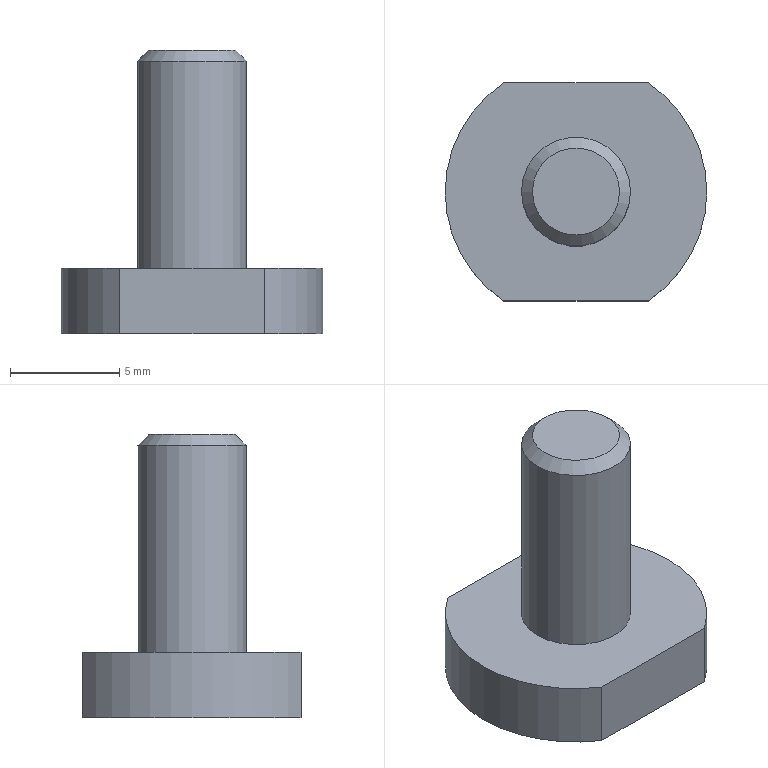Part | NX | 1 solid | 9 faces | box 12 x 10 x 13 mm | volume 506.8 mm3 | plane 5 | cylinder 3 | cone 1 | commonest cylinder face diameters 12 x2 5 x1
STEP:
#1=CARTESIAN_POINT('',(2.5,0.,3.));
#2=VERTEX_POINT('',#1);
#3=CARTESIAN_POINT('',(0.,0.,3.));
#4=DIRECTION('',(0.,0.,1.));
#5=DIRECTION('',(1.,0.,0.));
#6=AXIS2_PLACEMENT_3D('',#3,#4,#5);
#7=CIRCLE('',#6,2.5);
#8=EDGE_CURVE('',#2,#2,#7,.T.);
#9=ORIENTED_EDGE('',*,*,#8,.F.);
#10=EDGE_LOOP('',(#9));
#11=FACE_BOUND('',#10,.T.);
#12=CARTESIAN_POINT('',(-3.317,5.,3.));
#13=VERTEX_POINT('',#12);
#14=CARTESIAN_POINT('',(-3.317,-5.,3.));
#15=VERTEX_POINT('',#14);
#16=CARTESIAN_POINT('',(0.,0.,3.));
#17=DIRECTION('',(0.,0.,1.));
#18=DIRECTION('',(1.,0.,0.));
#19=AXIS2_PLACEMENT_3D('',#16,#17,#18);
#20=CIRCLE('',#19,6.);
#21=EDGE_CURVE('',#13,#15,#20,.T.);
#22=ORIENTED_EDGE('',*,*,#21,.T.);
#23=CARTESIAN_POINT('',(3.317,-5.,3.));
#24=VERTEX_POINT('',#23);
#25=CARTESIAN_POINT('',(0.,-5.,3.));
#26=DIRECTION('',(1.,0.,0.));
#27=VECTOR('',#26,1000.);
#28=LINE('',#25,#27);
#29=EDGE_CURVE('',#15,#24,#28,.T.);
#30=ORIENTED_EDGE('',*,*,#29,.T.);
#31=CARTESIAN_POINT('',(3.317,5.,3.));
#32=VERTEX_POINT('',#31);
#33=CARTESIAN_POINT('',(0.,0.,3.));
#34=DIRECTION('',(0.,0.,1.));
#35=DIRECTION('',(1.,0.,0.));
#36=AXIS2_PLACEMENT_3D('',#33,#34,#35);
#37=CIRCLE('',#36,6.);
#38=EDGE_CURVE('',#24,#32,#37,.T.);
#39=ORIENTED_EDGE('',*,*,#38,.T.);
#40=CARTESIAN_POINT('',(0.,5.,3.));
#41=DIRECTION('',(-1.,0.,0.));
#42=VECTOR('',#41,1000.);
#43=LINE('',#40,#42);
#44=EDGE_CURVE('',#32,#13,#43,.T.);
#45=ORIENTED_EDGE('',*,*,#44,.T.);
#46=EDGE_LOOP('',(#22,#30,#39,#45));
#47=FACE_BOUND('',#46,.T.);
#48=CARTESIAN_POINT('',(0.,0.,3.));
#49=DIRECTION('',(0.,0.,1.));
#50=DIRECTION('',(1.,0.,0.));
#51=AXIS2_PLACEMENT_3D('',#48,#49,#50);
#52=PLANE('',#51);
#53=ADVANCED_FACE('',(#11,#47),#52,.T.);
#54=CARTESIAN_POINT('',(-3.317,-5.,0.));
#55=VERTEX_POINT('',#54);
#56=CARTESIAN_POINT('',(-3.317,-5.,3.));
#57=DIRECTION('',(0.,0.,-1.));
#58=VECTOR('',#57,1000.);
#59=LINE('',#56,#58);
#60=EDGE_CURVE('',#15,#55,#59,.T.);
#61=ORIENTED_EDGE('',*,*,#60,.F.);
#62=ORIENTED_EDGE('',*,*,#21,.F.);
#63=CARTESIAN_POINT('',(-3.317,5.,0.));
#64=VERTEX_POINT('',#63);
#65=CARTESIAN_POINT('',(-3.317,5.,3.));
#66=DIRECTION('',(0.,0.,-1.));
#67=VECTOR('',#66,1000.);
#68=LINE('',#65,#67);
#69=EDGE_CURVE('',#64,#13,#68,.F.);
#70=ORIENTED_EDGE('',*,*,#69,.F.);
#71=CARTESIAN_POINT('',(0.,0.,0.));
#72=DIRECTION('',(0.,0.,1.));
#73=DIRECTION('',(1.,0.,0.));
#74=AXIS2_PLACEMENT_3D('',#71,#72,#73);
#75=CIRCLE('',#74,6.);
#76=EDGE_CURVE('',#64,#55,#75,.T.);
#77=ORIENTED_EDGE('',*,*,#76,.T.);
#78=EDGE_LOOP('',(#61,#62,#70,#77));
#79=FACE_BOUND('',#78,.T.);
#80=CARTESIAN_POINT('',(0.,0.,3.));
#81=DIRECTION('',(0.,0.,-1.));
#82=DIRECTION('',(-1.,0.,0.));
#83=AXIS2_PLACEMENT_3D('',#80,#81,#82);
#84=CYLINDRICAL_SURFACE('',#83,6.);
#85=ADVANCED_FACE('',(#79),#84,.T.);
#86=CARTESIAN_POINT('',(3.317,-5.,0.));
#87=VERTEX_POINT('',#86);
#88=CARTESIAN_POINT('',(3.317,-5.,3.));
#89=DIRECTION('',(0.,0.,-1.));
#90=VECTOR('',#89,1000.);
#91=LINE('',#88,#90);
#92=EDGE_CURVE('',#87,#24,#91,.F.);
#93=ORIENTED_EDGE('',*,*,#92,.F.);
#94=CARTESIAN_POINT('',(3.317,5.,0.));
#95=VERTEX_POINT('',#94);
#96=CARTESIAN_POINT('',(0.,0.,0.));
#97=DIRECTION('',(0.,0.,1.));
#98=DIRECTION('',(1.,0.,0.));
#99=AXIS2_PLACEMENT_3D('',#96,#97,#98);
#100=CIRCLE('',#99,6.);
#101=EDGE_CURVE('',#87,#95,#100,.T.);
#102=ORIENTED_EDGE('',*,*,#101,.T.);
#103=CARTESIAN_POINT('',(3.317,5.,3.));
#104=DIRECTION('',(0.,0.,-1.));
#105=VECTOR('',#104,1000.);
#106=LINE('',#103,#105);
#107=EDGE_CURVE('',#32,#95,#106,.T.);
#108=ORIENTED_EDGE('',*,*,#107,.F.);
#109=ORIENTED_EDGE('',*,*,#38,.F.);
#110=EDGE_LOOP('',(#93,#102,#108,#109));
#111=FACE_BOUND('',#110,.T.);
#112=CARTESIAN_POINT('',(0.,0.,3.));
#113=DIRECTION('',(0.,0.,-1.));
#114=DIRECTION('',(-1.,0.,0.));
#115=AXIS2_PLACEMENT_3D('',#112,#113,#114);
#116=CYLINDRICAL_SURFACE('',#115,6.);
#117=ADVANCED_FACE('',(#111),#116,.T.);
#118=CARTESIAN_POINT('',(0.,-5.,0.));
#119=DIRECTION('',(1.,0.,0.));
#120=VECTOR('',#119,1000.);
#121=LINE('',#118,#120);
#122=EDGE_CURVE('',#55,#87,#121,.T.);
#123=ORIENTED_EDGE('',*,*,#122,.F.);
#124=ORIENTED_EDGE('',*,*,#76,.F.);
#125=CARTESIAN_POINT('',(0.,5.,0.));
#126=DIRECTION('',(-1.,0.,0.));
#127=VECTOR('',#126,1000.);
#128=LINE('',#125,#127);
#129=EDGE_CURVE('',#95,#64,#128,.T.);
#130=ORIENTED_EDGE('',*,*,#129,.F.);
#131=ORIENTED_EDGE('',*,*,#101,.F.);
#132=EDGE_LOOP('',(#123,#124,#130,#131));
#133=FACE_BOUND('',#132,.T.);
#134=CARTESIAN_POINT('',(0.,0.,0.));
#135=DIRECTION('',(0.,0.,1.));
#136=DIRECTION('',(1.,0.,0.));
#137=AXIS2_PLACEMENT_3D('',#134,#135,#136);
#138=PLANE('',#137);
#139=ADVANCED_FACE('',(#133),#138,.F.);
#140=CARTESIAN_POINT('',(2.5,0.,12.5));
#141=VERTEX_POINT('',#140);
#142=CARTESIAN_POINT('',(0.,0.,12.5));
#143=DIRECTION('',(0.,0.,1.));
#144=DIRECTION('',(1.,0.,0.));
#145=AXIS2_PLACEMENT_3D('',#142,#143,#144);
#146=CIRCLE('',#145,2.5);
#147=EDGE_CURVE('',#141,#141,#146,.F.);
#148=ORIENTED_EDGE('',*,*,#147,.T.);
#149=EDGE_LOOP('',(#148));
#150=FACE_BOUND('',#149,.T.);
#151=ORIENTED_EDGE('',*,*,#8,.T.);
#152=EDGE_LOOP('',(#151));
#153=FACE_BOUND('',#152,.T.);
#154=CARTESIAN_POINT('',(0.,0.,13.));
#155=DIRECTION('',(0.,0.,-1.));
#156=DIRECTION('',(-1.,0.,0.));
#157=AXIS2_PLACEMENT_3D('',#154,#155,#156);
#158=CYLINDRICAL_SURFACE('',#157,2.5);
#159=ADVANCED_FACE('',(#150,#153),#158,.T.);
#160=CARTESIAN_POINT('',(2.,0.,13.));
#161=VERTEX_POINT('',#160);
#162=CARTESIAN_POINT('',(0.,0.,13.));
#163=DIRECTION('',(0.,0.,1.));
#164=DIRECTION('',(1.,0.,0.));
#165=AXIS2_PLACEMENT_3D('',#162,#163,#164);
#166=CIRCLE('',#165,2.);
#167=EDGE_CURVE('',#161,#161,#166,.T.);
#168=ORIENTED_EDGE('',*,*,#167,.T.);
#169=EDGE_LOOP('',(#168));
#170=FACE_BOUND('',#169,.T.);
#171=CARTESIAN_POINT('',(0.,0.,13.));
#172=DIRECTION('',(0.,0.,1.));
#173=DIRECTION('',(1.,0.,0.));
#174=AXIS2_PLACEMENT_3D('',#171,#172,#173);
#175=PLANE('',#174);
#176=ADVANCED_FACE('',(#170),#175,.T.);
#177=ORIENTED_EDGE('',*,*,#107,.T.);
#178=ORIENTED_EDGE('',*,*,#129,.T.);
#179=ORIENTED_EDGE('',*,*,#69,.T.);
#180=ORIENTED_EDGE('',*,*,#44,.F.);
#181=EDGE_LOOP('',(#177,#178,#179,#180));
#182=FACE_BOUND('',#181,.T.);
#183=CARTESIAN_POINT('',(10.025,5.,13.));
#184=DIRECTION('',(0.,1.,0.));
#185=DIRECTION('',(0.,0.,1.));
#186=AXIS2_PLACEMENT_3D('',#183,#184,#185);
#187=PLANE('',#186);
#188=ADVANCED_FACE('',(#182),#187,.T.);
#189=ORIENTED_EDGE('',*,*,#60,.T.);
#190=ORIENTED_EDGE('',*,*,#122,.T.);
#191=ORIENTED_EDGE('',*,*,#92,.T.);
#192=ORIENTED_EDGE('',*,*,#29,.F.);
#193=EDGE_LOOP('',(#189,#190,#191,#192));
#194=FACE_BOUND('',#193,.T.);
#195=CARTESIAN_POINT('',(10.025,-5.,13.));
#196=DIRECTION('',(0.,-1.,0.));
#197=DIRECTION('',(1.,0.,0.));
#198=AXIS2_PLACEMENT_3D('',#195,#196,#197);
#199=PLANE('',#198);
#200=ADVANCED_FACE('',(#194),#199,.T.);
#201=ORIENTED_EDGE('',*,*,#147,.F.);
#202=EDGE_LOOP('',(#201));
#203=FACE_BOUND('',#202,.T.);
#204=ORIENTED_EDGE('',*,*,#167,.F.);
#205=EDGE_LOOP('',(#204));
#206=FACE_BOUND('',#205,.T.);
#207=CARTESIAN_POINT('',(0.,0.,13.));
#208=DIRECTION('',(0.,0.,-1.));
#209=DIRECTION('',(-1.,0.,0.));
#210=AXIS2_PLACEMENT_3D('',#207,#208,#209);
#211=CONICAL_SURFACE('',#210,2.,0.7854);
#212=ADVANCED_FACE('',(#203,#206),#211,.T.);
#213=CLOSED_SHELL('',(#53,#85,#117,#139,#159,#176,#188,#200,#212));
#214=MANIFOLD_SOLID_BREP('',#213);
#215=(LENGTH_UNIT()NAMED_UNIT(*)SI_UNIT(.MILLI.,.METRE.));
#216=UNCERTAINTY_MEASURE_WITH_UNIT(LENGTH_MEASURE(0.00001),#215,'','');
#217=(NAMED_UNIT(*)PLANE_ANGLE_UNIT()SI_UNIT($,.RADIAN.));
#218=(NAMED_UNIT(*)SI_UNIT($,.STERADIAN.)SOLID_ANGLE_UNIT());
#219=(GEOMETRIC_REPRESENTATION_CONTEXT(3)GLOBAL_UNCERTAINTY_ASSIGNED_CONTEXT((#216))GLOBAL_UNIT_ASSIGNED_CONTEXT((#215,#217,#218))REPRESENTATION_CONTEXT('',''));
#220=ADVANCED_BREP_SHAPE_REPRESENTATION('',(#214),#219);